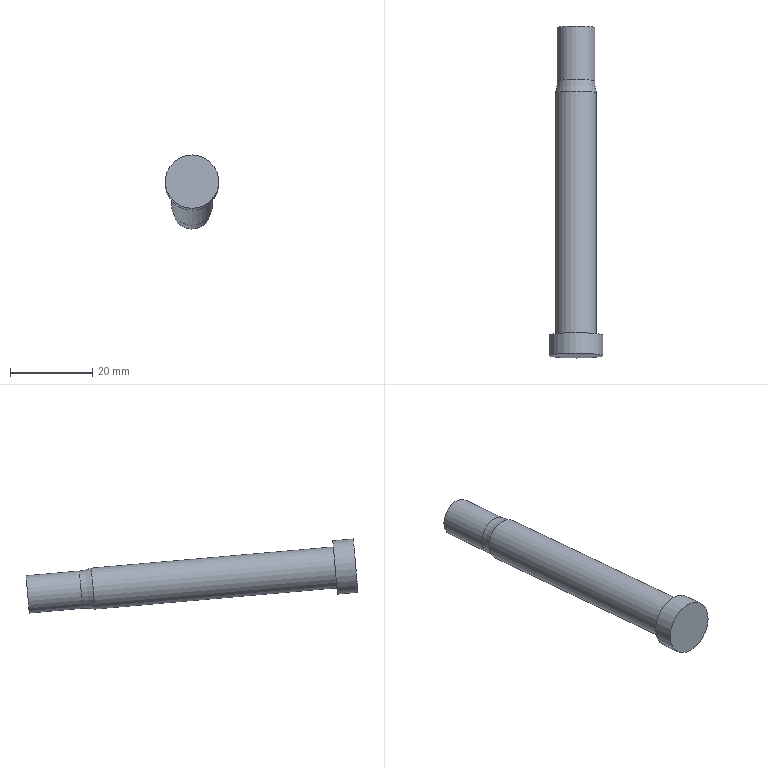Part | NX | features SPAS 10-80-9.100 2 | 1 solid | 7 faces | box 13 x 80.659 x 17.98 mm | volume 6352 mm3 | plane 3 | cylinder 3 | torus 1 | commonest cylinder face diameters 9.1 x1 10 x1 13 x1
STEP:
#1=CARTESIAN_POINT('',(198.727,-41.785,-52.211));
#2=VERTEX_POINT('',#1);
#3=CARTESIAN_POINT('',(198.727,-41.388,-47.678));
#4=DIRECTION('',(0.,-0.9962,0.08716));
#5=DIRECTION('',(0.,-0.08716,-0.9962));
#6=AXIS2_PLACEMENT_3D('',#3,#4,#5);
#7=CIRCLE('',#6,4.55);
#8=EDGE_CURVE('',#2,#2,#7,.T.);
#9=ORIENTED_EDGE('',*,*,#8,.F.);
#10=EDGE_LOOP('',(#9));
#11=FACE_BOUND('',#10,.T.);
#12=CARTESIAN_POINT('',(198.727,-41.388,-47.678));
#13=DIRECTION('',(0.,0.9962,-0.08716));
#14=DIRECTION('',(0.,0.08716,0.9962));
#15=AXIS2_PLACEMENT_3D('',#12,#13,#14);
#16=PLANE('',#15);
#17=ADVANCED_FACE('',(#11),#16,.T.);
#18=CARTESIAN_POINT('',(198.727,-54.735,-51.078));
#19=VERTEX_POINT('',#18);
#20=CARTESIAN_POINT('',(198.727,-54.339,-46.545));
#21=DIRECTION('',(0.,-0.9962,0.08716));
#22=DIRECTION('',(0.,-0.08716,-0.9962));
#23=AXIS2_PLACEMENT_3D('',#20,#21,#22);
#24=CIRCLE('',#23,4.55);
#25=EDGE_CURVE('',#19,#19,#24,.F.);
#26=ORIENTED_EDGE('',*,*,#25,.T.);
#27=EDGE_LOOP('',(#26));
#28=FACE_BOUND('',#27,.T.);
#29=ORIENTED_EDGE('',*,*,#8,.T.);
#30=EDGE_LOOP('',(#29));
#31=FACE_BOUND('',#30,.T.);
#32=CARTESIAN_POINT('',(198.727,-41.388,-47.678));
#33=DIRECTION('',(0.,-0.9962,0.08716));
#34=DIRECTION('',(0.,-0.08716,-0.9962));
#35=AXIS2_PLACEMENT_3D('',#32,#33,#34);
#36=CYLINDRICAL_SURFACE('',#35,4.55);
#37=ADVANCED_FACE('',(#28,#31),#36,.T.);
#38=CARTESIAN_POINT('',(198.727,-115.667,-36.161));
#39=VERTEX_POINT('',#38);
#40=CARTESIAN_POINT('',(198.727,-116.103,-41.142));
#41=DIRECTION('',(0.,0.9962,-0.08716));
#42=DIRECTION('',(0.,0.08716,0.9962));
#43=AXIS2_PLACEMENT_3D('',#40,#41,#42);
#44=CIRCLE('',#43,5.);
#45=EDGE_CURVE('',#39,#39,#44,.F.);
#46=ORIENTED_EDGE('',*,*,#45,.F.);
#47=EDGE_LOOP('',(#46));
#48=FACE_BOUND('',#47,.T.);
#49=CARTESIAN_POINT('',(198.727,-57.729,-51.268));
#50=VERTEX_POINT('',#49);
#51=CARTESIAN_POINT('',(198.727,-57.293,-46.287));
#52=DIRECTION('',(0.,-0.9962,0.08716));
#53=DIRECTION('',(0.,-0.08716,-0.9962));
#54=AXIS2_PLACEMENT_3D('',#51,#52,#53);
#55=CIRCLE('',#54,5.);
#56=EDGE_CURVE('',#50,#50,#55,.T.);
#57=ORIENTED_EDGE('',*,*,#56,.T.);
#58=EDGE_LOOP('',(#57));
#59=FACE_BOUND('',#58,.T.);
#60=CARTESIAN_POINT('',(198.727,-57.293,-46.287));
#61=DIRECTION('',(0.,-0.9962,0.08716));
#62=DIRECTION('',(0.,-0.08716,-0.9962));
#63=AXIS2_PLACEMENT_3D('',#60,#61,#62);
#64=CYLINDRICAL_SURFACE('',#63,5.);
#65=ADVANCED_FACE('',(#48,#59),#64,.T.);
#66=CARTESIAN_POINT('',(198.727,-121.65,-47.181));
#67=VERTEX_POINT('',#66);
#68=CARTESIAN_POINT('',(198.727,-121.084,-40.706));
#69=DIRECTION('',(0.,-0.9962,0.08716));
#70=DIRECTION('',(0.,-0.08716,-0.9962));
#71=AXIS2_PLACEMENT_3D('',#68,#69,#70);
#72=CIRCLE('',#71,6.5);
#73=EDGE_CURVE('',#67,#67,#72,.F.);
#74=ORIENTED_EDGE('',*,*,#73,.F.);
#75=EDGE_LOOP('',(#74));
#76=FACE_BOUND('',#75,.T.);
#77=CARTESIAN_POINT('',(198.727,-121.084,-40.706));
#78=DIRECTION('',(0.,-0.9962,0.08716));
#79=DIRECTION('',(0.,-0.08716,-0.9962));
#80=AXIS2_PLACEMENT_3D('',#77,#78,#79);
#81=PLANE('',#80);
#82=ADVANCED_FACE('',(#76),#81,.T.);
#83=ORIENTED_EDGE('',*,*,#45,.T.);
#84=EDGE_LOOP('',(#83));
#85=FACE_BOUND('',#84,.T.);
#86=CARTESIAN_POINT('',(198.727,-115.536,-34.667));
#87=VERTEX_POINT('',#86);
#88=CARTESIAN_POINT('',(198.727,-116.103,-41.142));
#89=DIRECTION('',(0.,0.9962,-0.08716));
#90=DIRECTION('',(0.,0.08716,0.9962));
#91=AXIS2_PLACEMENT_3D('',#88,#89,#90);
#92=CIRCLE('',#91,6.5);
#93=EDGE_CURVE('',#87,#87,#92,.F.);
#94=ORIENTED_EDGE('',*,*,#93,.F.);
#95=EDGE_LOOP('',(#94));
#96=FACE_BOUND('',#95,.T.);
#97=CARTESIAN_POINT('',(198.727,-116.103,-41.142));
#98=DIRECTION('',(0.,0.9962,-0.08716));
#99=DIRECTION('',(0.,0.08716,0.9962));
#100=AXIS2_PLACEMENT_3D('',#97,#98,#99);
#101=PLANE('',#100);
#102=ADVANCED_FACE('',(#85,#96),#101,.T.);
#103=ORIENTED_EDGE('',*,*,#73,.T.);
#104=EDGE_LOOP('',(#103));
#105=FACE_BOUND('',#104,.T.);
#106=ORIENTED_EDGE('',*,*,#93,.T.);
#107=EDGE_LOOP('',(#106));
#108=FACE_BOUND('',#107,.T.);
#109=CARTESIAN_POINT('',(198.727,-116.103,-41.142));
#110=DIRECTION('',(0.,-0.9962,0.08716));
#111=DIRECTION('',(0.,-0.08716,-0.9962));
#112=AXIS2_PLACEMENT_3D('',#109,#110,#111);
#113=CYLINDRICAL_SURFACE('',#112,6.5);
#114=ADVANCED_FACE('',(#105,#108),#113,.T.);
#115=ORIENTED_EDGE('',*,*,#25,.F.);
#116=EDGE_LOOP('',(#115));
#117=FACE_BOUND('',#116,.T.);
#118=ORIENTED_EDGE('',*,*,#56,.F.);
#119=EDGE_LOOP('',(#118));
#120=FACE_BOUND('',#119,.T.);
#121=CARTESIAN_POINT('',(198.727,-54.339,-46.545));
#122=DIRECTION('',(0.,-0.9962,0.08716));
#123=DIRECTION('',(0.,-0.08716,-0.9962));
#124=AXIS2_PLACEMENT_3D('',#121,#122,#123);
#125=TOROIDAL_SURFACE('',#124,14.55,10.);
#126=ADVANCED_FACE('',(#117,#120),#125,.F.);
#127=CLOSED_SHELL('',(#17,#37,#65,#82,#102,#114,#126));
#128=MANIFOLD_SOLID_BREP('',#127);
#129=(LENGTH_UNIT()NAMED_UNIT(*)SI_UNIT(.MILLI.,.METRE.));
#130=UNCERTAINTY_MEASURE_WITH_UNIT(LENGTH_MEASURE(0.00001),#129,'','');
#131=(NAMED_UNIT(*)PLANE_ANGLE_UNIT()SI_UNIT($,.RADIAN.));
#132=(NAMED_UNIT(*)SI_UNIT($,.STERADIAN.)SOLID_ANGLE_UNIT());
#133=(GEOMETRIC_REPRESENTATION_CONTEXT(3)GLOBAL_UNCERTAINTY_ASSIGNED_CONTEXT((#130))GLOBAL_UNIT_ASSIGNED_CONTEXT((#129,#131,#132))REPRESENTATION_CONTEXT('',''));
#134=ADVANCED_BREP_SHAPE_REPRESENTATION('',(#128),#133);